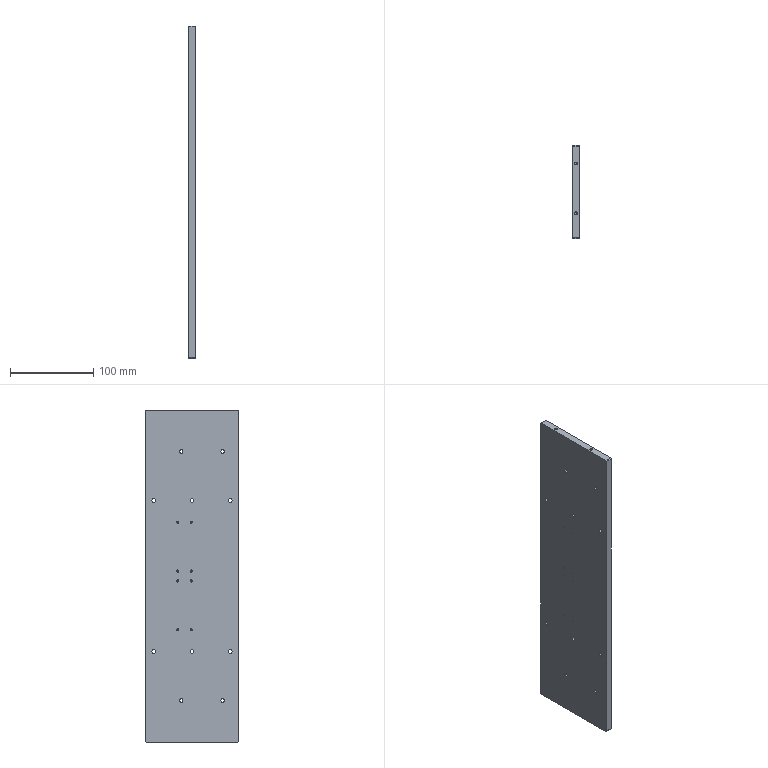Part | NX | 1 solid | 56 faces | box 8 x 112 x 400 mm | volume 355078 mm3 | cylinder 32 | plane 16 | cone 8 | commonest cylinder face diameters 2.5 x8 3.3 x8 4.5 x6 8 x6 4.2 x4
STEP:
#1=CARTESIAN_POINT('',(4.,1.,-4.75));
#2=VERTEX_POINT('',#1);
#3=CARTESIAN_POINT('',(4.,1.,-6.));
#4=DIRECTION('',(-1.,0.,0.));
#5=DIRECTION('',(0.,0.,1.));
#6=AXIS2_PLACEMENT_3D('',#3,#4,#5);
#7=CIRCLE('',#6,1.25);
#8=EDGE_CURVE('',#2,#2,#7,.T.);
#9=ORIENTED_EDGE('',*,*,#8,.T.);
#10=EDGE_LOOP('',(#9));
#11=FACE_BOUND('',#10,.T.);
#12=CARTESIAN_POINT('',(4.,17.,-4.75));
#13=VERTEX_POINT('',#12);
#14=CARTESIAN_POINT('',(4.,17.,-6.));
#15=DIRECTION('',(-1.,0.,0.));
#16=DIRECTION('',(0.,0.,1.));
#17=AXIS2_PLACEMENT_3D('',#14,#15,#16);
#18=CIRCLE('',#17,1.25);
#19=EDGE_CURVE('',#13,#13,#18,.T.);
#20=ORIENTED_EDGE('',*,*,#19,.T.);
#21=EDGE_LOOP('',(#20));
#22=FACE_BOUND('',#21,.T.);
#23=CARTESIAN_POINT('',(4.,17.,7.25));
#24=VERTEX_POINT('',#23);
#25=CARTESIAN_POINT('',(4.,17.,6.));
#26=DIRECTION('',(-1.,0.,0.));
#27=DIRECTION('',(0.,0.,1.));
#28=AXIS2_PLACEMENT_3D('',#25,#26,#27);
#29=CIRCLE('',#28,1.25);
#30=EDGE_CURVE('',#24,#24,#29,.T.);
#31=ORIENTED_EDGE('',*,*,#30,.T.);
#32=EDGE_LOOP('',(#31));
#33=FACE_BOUND('',#32,.T.);
#34=CARTESIAN_POINT('',(4.,1.,7.25));
#35=VERTEX_POINT('',#34);
#36=CARTESIAN_POINT('',(4.,1.,6.));
#37=DIRECTION('',(-1.,0.,0.));
#38=DIRECTION('',(0.,0.,1.));
#39=AXIS2_PLACEMENT_3D('',#36,#37,#38);
#40=CIRCLE('',#39,1.25);
#41=EDGE_CURVE('',#35,#35,#40,.T.);
#42=ORIENTED_EDGE('',*,*,#41,.T.);
#43=EDGE_LOOP('',(#42));
#44=FACE_BOUND('',#43,.T.);
#45=CARTESIAN_POINT('',(4.,17.,-63.75));
#46=VERTEX_POINT('',#45);
#47=CARTESIAN_POINT('',(4.,17.,-65.));
#48=DIRECTION('',(-1.,0.,0.));
#49=DIRECTION('',(0.,0.,1.));
#50=AXIS2_PLACEMENT_3D('',#47,#48,#49);
#51=CIRCLE('',#50,1.25);
#52=EDGE_CURVE('',#46,#46,#51,.T.);
#53=ORIENTED_EDGE('',*,*,#52,.T.);
#54=EDGE_LOOP('',(#53));
#55=FACE_BOUND('',#54,.T.);
#56=CARTESIAN_POINT('',(4.,1.,-63.75));
#57=VERTEX_POINT('',#56);
#58=CARTESIAN_POINT('',(4.,1.,-65.));
#59=DIRECTION('',(-1.,0.,0.));
#60=DIRECTION('',(0.,0.,1.));
#61=AXIS2_PLACEMENT_3D('',#58,#59,#60);
#62=CIRCLE('',#61,1.25);
#63=EDGE_CURVE('',#57,#57,#62,.T.);
#64=ORIENTED_EDGE('',*,*,#63,.T.);
#65=EDGE_LOOP('',(#64));
#66=FACE_BOUND('',#65,.T.);
#67=CARTESIAN_POINT('',(4.,1.,66.25));
#68=VERTEX_POINT('',#67);
#69=CARTESIAN_POINT('',(4.,1.,65.));
#70=DIRECTION('',(-1.,0.,0.));
#71=DIRECTION('',(0.,0.,1.));
#72=AXIS2_PLACEMENT_3D('',#69,#70,#71);
#73=CIRCLE('',#72,1.25);
#74=EDGE_CURVE('',#68,#68,#73,.T.);
#75=ORIENTED_EDGE('',*,*,#74,.T.);
#76=EDGE_LOOP('',(#75));
#77=FACE_BOUND('',#76,.T.);
#78=CARTESIAN_POINT('',(4.,17.,66.25));
#79=VERTEX_POINT('',#78);
#80=CARTESIAN_POINT('',(4.,17.,65.));
#81=DIRECTION('',(-1.,0.,0.));
#82=DIRECTION('',(0.,0.,1.));
#83=AXIS2_PLACEMENT_3D('',#80,#81,#82);
#84=CIRCLE('',#83,1.25);
#85=EDGE_CURVE('',#79,#79,#84,.T.);
#86=ORIENTED_EDGE('',*,*,#85,.T.);
#87=EDGE_LOOP('',(#86));
#88=FACE_BOUND('',#87,.T.);
#89=CARTESIAN_POINT('',(4.,46.,87.));
#90=VERTEX_POINT('',#89);
#91=CARTESIAN_POINT('',(4.,46.,91.));
#92=DIRECTION('',(1.,0.,0.));
#93=DIRECTION('',(0.,0.,-1.));
#94=AXIS2_PLACEMENT_3D('',#91,#92,#93);
#95=CIRCLE('',#94,4.);
#96=EDGE_CURVE('',#90,#90,#95,.T.);
#97=ORIENTED_EDGE('',*,*,#96,.F.);
#98=EDGE_LOOP('',(#97));
#99=FACE_BOUND('',#98,.T.);
#100=CARTESIAN_POINT('',(4.,0.,87.));
#101=VERTEX_POINT('',#100);
#102=CARTESIAN_POINT('',(4.,0.,91.));
#103=DIRECTION('',(1.,0.,0.));
#104=DIRECTION('',(0.,0.,-1.));
#105=AXIS2_PLACEMENT_3D('',#102,#103,#104);
#106=CIRCLE('',#105,4.);
#107=EDGE_CURVE('',#101,#101,#106,.T.);
#108=ORIENTED_EDGE('',*,*,#107,.F.);
#109=EDGE_LOOP('',(#108));
#110=FACE_BOUND('',#109,.T.);
#111=CARTESIAN_POINT('',(4.,-46.,87.));
#112=VERTEX_POINT('',#111);
#113=CARTESIAN_POINT('',(4.,-46.,91.));
#114=DIRECTION('',(1.,0.,0.));
#115=DIRECTION('',(0.,0.,-1.));
#116=AXIS2_PLACEMENT_3D('',#113,#114,#115);
#117=CIRCLE('',#116,4.);
#118=EDGE_CURVE('',#112,#112,#117,.T.);
#119=ORIENTED_EDGE('',*,*,#118,.F.);
#120=EDGE_LOOP('',(#119));
#121=FACE_BOUND('',#120,.T.);
#122=CARTESIAN_POINT('',(4.,46.,-95.));
#123=VERTEX_POINT('',#122);
#124=CARTESIAN_POINT('',(4.,46.,-91.));
#125=DIRECTION('',(1.,0.,0.));
#126=DIRECTION('',(0.,0.,-1.));
#127=AXIS2_PLACEMENT_3D('',#124,#125,#126);
#128=CIRCLE('',#127,4.);
#129=EDGE_CURVE('',#123,#123,#128,.T.);
#130=ORIENTED_EDGE('',*,*,#129,.F.);
#131=EDGE_LOOP('',(#130));
#132=FACE_BOUND('',#131,.T.);
#133=CARTESIAN_POINT('',(4.,0.,-95.));
#134=VERTEX_POINT('',#133);
#135=CARTESIAN_POINT('',(4.,0.,-91.));
#136=DIRECTION('',(1.,0.,0.));
#137=DIRECTION('',(0.,0.,-1.));
#138=AXIS2_PLACEMENT_3D('',#135,#136,#137);
#139=CIRCLE('',#138,4.);
#140=EDGE_CURVE('',#134,#134,#139,.T.);
#141=ORIENTED_EDGE('',*,*,#140,.F.);
#142=EDGE_LOOP('',(#141));
#143=FACE_BOUND('',#142,.T.);
#144=CARTESIAN_POINT('',(4.,-46.,-95.));
#145=VERTEX_POINT('',#144);
#146=CARTESIAN_POINT('',(4.,-46.,-91.));
#147=DIRECTION('',(1.,0.,0.));
#148=DIRECTION('',(0.,0.,-1.));
#149=AXIS2_PLACEMENT_3D('',#146,#147,#148);
#150=CIRCLE('',#149,4.);
#151=EDGE_CURVE('',#145,#145,#150,.T.);
#152=ORIENTED_EDGE('',*,*,#151,.F.);
#153=EDGE_LOOP('',(#152));
#154=FACE_BOUND('',#153,.T.);
#155=CARTESIAN_POINT('',(4.,13.,-147.9));
#156=VERTEX_POINT('',#155);
#157=CARTESIAN_POINT('',(4.,13.,-150.));
#158=DIRECTION('',(-1.,0.,0.));
#159=DIRECTION('',(0.,0.,1.));
#160=AXIS2_PLACEMENT_3D('',#157,#158,#159);
#161=CIRCLE('',#160,2.1);
#162=EDGE_CURVE('',#156,#156,#161,.T.);
#163=ORIENTED_EDGE('',*,*,#162,.T.);
#164=EDGE_LOOP('',(#163));
#165=FACE_BOUND('',#164,.T.);
#166=CARTESIAN_POINT('',(4.,-37.,152.1));
#167=VERTEX_POINT('',#166);
#168=CARTESIAN_POINT('',(4.,-37.,150.));
#169=DIRECTION('',(-1.,0.,0.));
#170=DIRECTION('',(0.,0.,1.));
#171=AXIS2_PLACEMENT_3D('',#168,#169,#170);
#172=CIRCLE('',#171,2.1);
#173=EDGE_CURVE('',#167,#167,#172,.T.);
#174=ORIENTED_EDGE('',*,*,#173,.T.);
#175=EDGE_LOOP('',(#174));
#176=FACE_BOUND('',#175,.T.);
#177=CARTESIAN_POINT('',(4.,-37.,-147.9));
#178=VERTEX_POINT('',#177);
#179=CARTESIAN_POINT('',(4.,-37.,-150.));
#180=DIRECTION('',(-1.,0.,0.));
#181=DIRECTION('',(0.,0.,1.));
#182=AXIS2_PLACEMENT_3D('',#179,#180,#181);
#183=CIRCLE('',#182,2.1);
#184=EDGE_CURVE('',#178,#178,#183,.T.);
#185=ORIENTED_EDGE('',*,*,#184,.T.);
#186=EDGE_LOOP('',(#185));
#187=FACE_BOUND('',#186,.T.);
#188=CARTESIAN_POINT('',(4.,13.,152.1));
#189=VERTEX_POINT('',#188);
#190=CARTESIAN_POINT('',(4.,13.,150.));
#191=DIRECTION('',(-1.,0.,0.));
#192=DIRECTION('',(0.,0.,1.));
#193=AXIS2_PLACEMENT_3D('',#190,#191,#192);
#194=CIRCLE('',#193,2.1);
#195=EDGE_CURVE('',#189,#189,#194,.T.);
#196=ORIENTED_EDGE('',*,*,#195,.T.);
#197=EDGE_LOOP('',(#196));
#198=FACE_BOUND('',#197,.T.);
#199=CARTESIAN_POINT('',(4.,56.,199.));
#200=VERTEX_POINT('',#199);
#201=CARTESIAN_POINT('',(4.,56.,-199.));
#202=VERTEX_POINT('',#201);
#203=CARTESIAN_POINT('',(4.,56.,200.));
#204=DIRECTION('',(0.,0.,-1.));
#205=VECTOR('',#204,1000.);
#206=LINE('',#203,#205);
#207=EDGE_CURVE('',#200,#202,#206,.T.);
#208=ORIENTED_EDGE('',*,*,#207,.F.);
#209=CARTESIAN_POINT('',(4.,55.,200.));
#210=VERTEX_POINT('',#209);
#211=CARTESIAN_POINT('',(4.,55.,200.));
#212=DIRECTION('',(0.,-0.7071,0.7071));
#213=VECTOR('',#212,1000.);
#214=LINE('',#211,#213);
#215=EDGE_CURVE('',#200,#210,#214,.T.);
#216=ORIENTED_EDGE('',*,*,#215,.T.);
#217=CARTESIAN_POINT('',(4.,-55.,200.));
#218=VERTEX_POINT('',#217);
#219=CARTESIAN_POINT('',(4.,56.,200.));
#220=DIRECTION('',(0.,1.,0.));
#221=VECTOR('',#220,1000.);
#222=LINE('',#219,#221);
#223=EDGE_CURVE('',#218,#210,#222,.T.);
#224=ORIENTED_EDGE('',*,*,#223,.F.);
#225=CARTESIAN_POINT('',(4.,-56.,199.));
#226=VERTEX_POINT('',#225);
#227=CARTESIAN_POINT('',(4.,-55.,200.));
#228=DIRECTION('',(0.,-0.7071,-0.7071));
#229=VECTOR('',#228,1000.);
#230=LINE('',#227,#229);
#231=EDGE_CURVE('',#218,#226,#230,.T.);
#232=ORIENTED_EDGE('',*,*,#231,.T.);
#233=CARTESIAN_POINT('',(4.,-56.,-199.));
#234=VERTEX_POINT('',#233);
#235=CARTESIAN_POINT('',(4.,-56.,200.));
#236=DIRECTION('',(0.,0.,-1.));
#237=VECTOR('',#236,1000.);
#238=LINE('',#235,#237);
#239=EDGE_CURVE('',#226,#234,#238,.T.);
#240=ORIENTED_EDGE('',*,*,#239,.T.);
#241=CARTESIAN_POINT('',(4.,-55.,-200.));
#242=VERTEX_POINT('',#241);
#243=CARTESIAN_POINT('',(4.,-56.,-199.));
#244=DIRECTION('',(0.,-0.7071,0.7071));
#245=VECTOR('',#244,1000.);
#246=LINE('',#243,#245);
#247=EDGE_CURVE('',#234,#242,#246,.F.);
#248=ORIENTED_EDGE('',*,*,#247,.T.);
#249=CARTESIAN_POINT('',(4.,55.,-200.));
#250=VERTEX_POINT('',#249);
#251=CARTESIAN_POINT('',(4.,56.,-200.));
#252=DIRECTION('',(0.,1.,0.));
#253=VECTOR('',#252,1000.);
#254=LINE('',#251,#253);
#255=EDGE_CURVE('',#242,#250,#254,.T.);
#256=ORIENTED_EDGE('',*,*,#255,.T.);
#257=CARTESIAN_POINT('',(4.,56.,-199.));
#258=DIRECTION('',(0.,-0.7071,-0.7071));
#259=VECTOR('',#258,1000.);
#260=LINE('',#257,#259);
#261=EDGE_CURVE('',#250,#202,#260,.F.);
#262=ORIENTED_EDGE('',*,*,#261,.T.);
#263=EDGE_LOOP('',(#208,#216,#224,#232,#240,#248,#256,#262));
#264=FACE_BOUND('',#263,.T.);
#265=CARTESIAN_POINT('',(4.,56.,200.));
#266=DIRECTION('',(-1.,0.,0.));
#267=DIRECTION('',(0.,-1.,0.));
#268=AXIS2_PLACEMENT_3D('',#265,#266,#267);
#269=PLANE('',#268);
#270=ADVANCED_FACE('',(#11,#22,#33,#44,#55,#66,#77,#88,#99,#110,#121,#132,#143,#154,#165,#176,#187,#198,#264),#269,.F.);
#271=CARTESIAN_POINT('',(0.,56.,61.65));
#272=VERTEX_POINT('',#271);
#273=CARTESIAN_POINT('',(0.,56.,60.));
#274=DIRECTION('',(0.,1.,0.));
#275=DIRECTION('',(0.,0.,1.));
#276=AXIS2_PLACEMENT_3D('',#273,#274,#275);
#277=CIRCLE('',#276,1.65);
#278=EDGE_CURVE('',#272,#272,#277,.T.);
#279=ORIENTED_EDGE('',*,*,#278,.F.);
#280=EDGE_LOOP('',(#279));
#281=FACE_BOUND('',#280,.T.);
#282=CARTESIAN_POINT('',(0.,56.,181.65));
#283=VERTEX_POINT('',#282);
#284=CARTESIAN_POINT('',(0.,56.,180.));
#285=DIRECTION('',(0.,1.,0.));
#286=DIRECTION('',(0.,0.,1.));
#287=AXIS2_PLACEMENT_3D('',#284,#285,#286);
#288=CIRCLE('',#287,1.65);
#289=EDGE_CURVE('',#283,#283,#288,.T.);
#290=ORIENTED_EDGE('',*,*,#289,.F.);
#291=EDGE_LOOP('',(#290));
#292=FACE_BOUND('',#291,.T.);
#293=CARTESIAN_POINT('',(0.,56.,-58.35));
#294=VERTEX_POINT('',#293);
#295=CARTESIAN_POINT('',(0.,56.,-60.));
#296=DIRECTION('',(0.,1.,0.));
#297=DIRECTION('',(0.,0.,1.));
#298=AXIS2_PLACEMENT_3D('',#295,#296,#297);
#299=CIRCLE('',#298,1.65);
#300=EDGE_CURVE('',#294,#294,#299,.T.);
#301=ORIENTED_EDGE('',*,*,#300,.F.);
#302=EDGE_LOOP('',(#301));
#303=FACE_BOUND('',#302,.T.);
#304=CARTESIAN_POINT('',(0.,56.,-178.35));
#305=VERTEX_POINT('',#304);
#306=CARTESIAN_POINT('',(0.,56.,-180.));
#307=DIRECTION('',(0.,1.,0.));
#308=DIRECTION('',(0.,0.,1.));
#309=AXIS2_PLACEMENT_3D('',#306,#307,#308);
#310=CIRCLE('',#309,1.65);
#311=EDGE_CURVE('',#305,#305,#310,.T.);
#312=ORIENTED_EDGE('',*,*,#311,.F.);
#313=EDGE_LOOP('',(#312));
#314=FACE_BOUND('',#313,.T.);
#315=CARTESIAN_POINT('',(-4.,56.,199.));
#316=VERTEX_POINT('',#315);
#317=CARTESIAN_POINT('',(-4.,56.,-199.));
#318=VERTEX_POINT('',#317);
#319=CARTESIAN_POINT('',(-4.,56.,200.));
#320=DIRECTION('',(0.,0.,-1.));
#321=VECTOR('',#320,1000.);
#322=LINE('',#319,#321);
#323=EDGE_CURVE('',#316,#318,#322,.T.);
#324=ORIENTED_EDGE('',*,*,#323,.F.);
#325=CARTESIAN_POINT('',(4.,56.,199.));
#326=DIRECTION('',(1.,0.,0.));
#327=VECTOR('',#326,1000.);
#328=LINE('',#325,#327);
#329=EDGE_CURVE('',#316,#200,#328,.T.);
#330=ORIENTED_EDGE('',*,*,#329,.T.);
#331=ORIENTED_EDGE('',*,*,#207,.T.);
#332=CARTESIAN_POINT('',(-4.,56.,-199.));
#333=DIRECTION('',(-1.,0.,0.));
#334=VECTOR('',#333,1000.);
#335=LINE('',#332,#334);
#336=EDGE_CURVE('',#202,#318,#335,.T.);
#337=ORIENTED_EDGE('',*,*,#336,.T.);
#338=EDGE_LOOP('',(#324,#330,#331,#337));
#339=FACE_BOUND('',#338,.T.);
#340=CARTESIAN_POINT('',(-4.,56.,200.));
#341=DIRECTION('',(0.,-1.,0.));
#342=DIRECTION('',(0.,0.,-1.));
#343=AXIS2_PLACEMENT_3D('',#340,#341,#342);
#344=PLANE('',#343);
#345=ADVANCED_FACE('',(#281,#292,#303,#314,#339),#344,.F.);
#346=CARTESIAN_POINT('',(-4.,1.,-4.75));
#347=VERTEX_POINT('',#346);
#348=CARTESIAN_POINT('',(-4.,1.,-6.));
#349=DIRECTION('',(-1.,0.,0.));
#350=DIRECTION('',(0.,0.,1.));
#351=AXIS2_PLACEMENT_3D('',#348,#349,#350);
#352=CIRCLE('',#351,1.25);
#353=EDGE_CURVE('',#347,#347,#352,.T.);
#354=ORIENTED_EDGE('',*,*,#353,.F.);
#355=EDGE_LOOP('',(#354));
#356=FACE_BOUND('',#355,.T.);
#357=CARTESIAN_POINT('',(-4.,17.,-4.75));
#358=VERTEX_POINT('',#357);
#359=CARTESIAN_POINT('',(-4.,17.,-6.));
#360=DIRECTION('',(-1.,0.,0.));
#361=DIRECTION('',(0.,0.,1.));
#362=AXIS2_PLACEMENT_3D('',#359,#360,#361);
#363=CIRCLE('',#362,1.25);
#364=EDGE_CURVE('',#358,#358,#363,.T.);
#365=ORIENTED_EDGE('',*,*,#364,.F.);
#366=EDGE_LOOP('',(#365));
#367=FACE_BOUND('',#366,.T.);
#368=CARTESIAN_POINT('',(-4.,17.,7.25));
#369=VERTEX_POINT('',#368);
#370=CARTESIAN_POINT('',(-4.,17.,6.));
#371=DIRECTION('',(-1.,0.,0.));
#372=DIRECTION('',(0.,0.,1.));
#373=AXIS2_PLACEMENT_3D('',#370,#371,#372);
#374=CIRCLE('',#373,1.25);
#375=EDGE_CURVE('',#369,#369,#374,.T.);
#376=ORIENTED_EDGE('',*,*,#375,.F.);
#377=EDGE_LOOP('',(#376));
#378=FACE_BOUND('',#377,.T.);
#379=CARTESIAN_POINT('',(-4.,1.,7.25));
#380=VERTEX_POINT('',#379);
#381=CARTESIAN_POINT('',(-4.,1.,6.));
#382=DIRECTION('',(-1.,0.,0.));
#383=DIRECTION('',(0.,0.,1.));
#384=AXIS2_PLACEMENT_3D('',#381,#382,#383);
#385=CIRCLE('',#384,1.25);
#386=EDGE_CURVE('',#380,#380,#385,.T.);
#387=ORIENTED_EDGE('',*,*,#386,.F.);
#388=EDGE_LOOP('',(#387));
#389=FACE_BOUND('',#388,.T.);
#390=CARTESIAN_POINT('',(-4.,17.,-63.75));
#391=VERTEX_POINT('',#390);
#392=CARTESIAN_POINT('',(-4.,17.,-65.));
#393=DIRECTION('',(-1.,0.,0.));
#394=DIRECTION('',(0.,0.,1.));
#395=AXIS2_PLACEMENT_3D('',#392,#393,#394);
#396=CIRCLE('',#395,1.25);
#397=EDGE_CURVE('',#391,#391,#396,.T.);
#398=ORIENTED_EDGE('',*,*,#397,.F.);
#399=EDGE_LOOP('',(#398));
#400=FACE_BOUND('',#399,.T.);
#401=CARTESIAN_POINT('',(-4.,1.,-63.75));
#402=VERTEX_POINT('',#401);
#403=CARTESIAN_POINT('',(-4.,1.,-65.));
#404=DIRECTION('',(-1.,0.,0.));
#405=DIRECTION('',(0.,0.,1.));
#406=AXIS2_PLACEMENT_3D('',#403,#404,#405);
#407=CIRCLE('',#406,1.25);
#408=EDGE_CURVE('',#402,#402,#407,.T.);
#409=ORIENTED_EDGE('',*,*,#408,.F.);
#410=EDGE_LOOP('',(#409));
#411=FACE_BOUND('',#410,.T.);
#412=CARTESIAN_POINT('',(-4.,1.,66.25));
#413=VERTEX_POINT('',#412);
#414=CARTESIAN_POINT('',(-4.,1.,65.));
#415=DIRECTION('',(-1.,0.,0.));
#416=DIRECTION('',(0.,0.,1.));
#417=AXIS2_PLACEMENT_3D('',#414,#415,#416);
#418=CIRCLE('',#417,1.25);
#419=EDGE_CURVE('',#413,#413,#418,.T.);
#420=ORIENTED_EDGE('',*,*,#419,.F.);
#421=EDGE_LOOP('',(#420));
#422=FACE_BOUND('',#421,.T.);
#423=CARTESIAN_POINT('',(-4.,17.,66.25));
#424=VERTEX_POINT('',#423);
#425=CARTESIAN_POINT('',(-4.,17.,65.));
#426=DIRECTION('',(-1.,0.,0.));
#427=DIRECTION('',(0.,0.,1.));
#428=AXIS2_PLACEMENT_3D('',#425,#426,#427);
#429=CIRCLE('',#428,1.25);
#430=EDGE_CURVE('',#424,#424,#429,.T.);
#431=ORIENTED_EDGE('',*,*,#430,.F.);
#432=EDGE_LOOP('',(#431));
#433=FACE_BOUND('',#432,.T.);
#434=CARTESIAN_POINT('',(-4.,46.,88.75));
#435=VERTEX_POINT('',#434);
#436=CARTESIAN_POINT('',(-4.,46.,91.));
#437=DIRECTION('',(1.,0.,0.));
#438=DIRECTION('',(0.,0.,-1.));
#439=AXIS2_PLACEMENT_3D('',#436,#437,#438);
#440=CIRCLE('',#439,2.25);
#441=EDGE_CURVE('',#435,#435,#440,.T.);
#442=ORIENTED_EDGE('',*,*,#441,.T.);
#443=EDGE_LOOP('',(#442));
#444=FACE_BOUND('',#443,.T.);
#445=CARTESIAN_POINT('',(-4.,0.,88.75));
#446=VERTEX_POINT('',#445);
#447=CARTESIAN_POINT('',(-4.,0.,91.));
#448=DIRECTION('',(1.,0.,0.));
#449=DIRECTION('',(0.,0.,-1.));
#450=AXIS2_PLACEMENT_3D('',#447,#448,#449);
#451=CIRCLE('',#450,2.25);
#452=EDGE_CURVE('',#446,#446,#451,.T.);
#453=ORIENTED_EDGE('',*,*,#452,.T.);
#454=EDGE_LOOP('',(#453));
#455=FACE_BOUND('',#454,.T.);
#456=CARTESIAN_POINT('',(-4.,-46.,88.75));
#457=VERTEX_POINT('',#456);
#458=CARTESIAN_POINT('',(-4.,-46.,91.));
#459=DIRECTION('',(1.,0.,0.));
#460=DIRECTION('',(0.,0.,-1.));
#461=AXIS2_PLACEMENT_3D('',#458,#459,#460);
#462=CIRCLE('',#461,2.25);
#463=EDGE_CURVE('',#457,#457,#462,.T.);
#464=ORIENTED_EDGE('',*,*,#463,.T.);
#465=EDGE_LOOP('',(#464));
#466=FACE_BOUND('',#465,.T.);
#467=CARTESIAN_POINT('',(-4.,46.,-93.25));
#468=VERTEX_POINT('',#467);
#469=CARTESIAN_POINT('',(-4.,46.,-91.));
#470=DIRECTION('',(1.,0.,0.));
#471=DIRECTION('',(0.,0.,-1.));
#472=AXIS2_PLACEMENT_3D('',#469,#470,#471);
#473=CIRCLE('',#472,2.25);
#474=EDGE_CURVE('',#468,#468,#473,.T.);
#475=ORIENTED_EDGE('',*,*,#474,.T.);
#476=EDGE_LOOP('',(#475));
#477=FACE_BOUND('',#476,.T.);
#478=CARTESIAN_POINT('',(-4.,0.,-93.25));
#479=VERTEX_POINT('',#478);
#480=CARTESIAN_POINT('',(-4.,0.,-91.));
#481=DIRECTION('',(1.,0.,0.));
#482=DIRECTION('',(0.,0.,-1.));
#483=AXIS2_PLACEMENT_3D('',#480,#481,#482);
#484=CIRCLE('',#483,2.25);
#485=EDGE_CURVE('',#479,#479,#484,.T.);
#486=ORIENTED_EDGE('',*,*,#485,.T.);
#487=EDGE_LOOP('',(#486));
#488=FACE_BOUND('',#487,.T.);
#489=CARTESIAN_POINT('',(-4.,-46.,-93.25));
#490=VERTEX_POINT('',#489);
#491=CARTESIAN_POINT('',(-4.,-46.,-91.));
#492=DIRECTION('',(1.,0.,0.));
#493=DIRECTION('',(0.,0.,-1.));
#494=AXIS2_PLACEMENT_3D('',#491,#492,#493);
#495=CIRCLE('',#494,2.25);
#496=EDGE_CURVE('',#490,#490,#495,.T.);
#497=ORIENTED_EDGE('',*,*,#496,.T.);
#498=EDGE_LOOP('',(#497));
#499=FACE_BOUND('',#498,.T.);
#500=CARTESIAN_POINT('',(-4.,13.,-147.9));
#501=VERTEX_POINT('',#500);
#502=CARTESIAN_POINT('',(-4.,13.,-150.));
#503=DIRECTION('',(-1.,0.,0.));
#504=DIRECTION('',(0.,0.,1.));
#505=AXIS2_PLACEMENT_3D('',#502,#503,#504);
#506=CIRCLE('',#505,2.1);
#507=EDGE_CURVE('',#501,#501,#506,.T.);
#508=ORIENTED_EDGE('',*,*,#507,.F.);
#509=EDGE_LOOP('',(#508));
#510=FACE_BOUND('',#509,.T.);
#511=CARTESIAN_POINT('',(-4.,-37.,152.1));
#512=VERTEX_POINT('',#511);
#513=CARTESIAN_POINT('',(-4.,-37.,150.));
#514=DIRECTION('',(-1.,0.,0.));
#515=DIRECTION('',(0.,0.,1.));
#516=AXIS2_PLACEMENT_3D('',#513,#514,#515);
#517=CIRCLE('',#516,2.1);
#518=EDGE_CURVE('',#512,#512,#517,.T.);
#519=ORIENTED_EDGE('',*,*,#518,.F.);
#520=EDGE_LOOP('',(#519));
#521=FACE_BOUND('',#520,.T.);
#522=CARTESIAN_POINT('',(-4.,-37.,-147.9));
#523=VERTEX_POINT('',#522);
#524=CARTESIAN_POINT('',(-4.,-37.,-150.));
#525=DIRECTION('',(-1.,0.,0.));
#526=DIRECTION('',(0.,0.,1.));
#527=AXIS2_PLACEMENT_3D('',#524,#525,#526);
#528=CIRCLE('',#527,2.1);
#529=EDGE_CURVE('',#523,#523,#528,.T.);
#530=ORIENTED_EDGE('',*,*,#529,.F.);
#531=EDGE_LOOP('',(#530));
#532=FACE_BOUND('',#531,.T.);
#533=CARTESIAN_POINT('',(-4.,13.,152.1));
#534=VERTEX_POINT('',#533);
#535=CARTESIAN_POINT('',(-4.,13.,150.));
#536=DIRECTION('',(-1.,0.,0.));
#537=DIRECTION('',(0.,0.,1.));
#538=AXIS2_PLACEMENT_3D('',#535,#536,#537);
#539=CIRCLE('',#538,2.1);
#540=EDGE_CURVE('',#534,#534,#539,.T.);
#541=ORIENTED_EDGE('',*,*,#540,.F.);
#542=EDGE_LOOP('',(#541));
#543=FACE_BOUND('',#542,.T.);
#544=CARTESIAN_POINT('',(-4.,55.,200.));
#545=VERTEX_POINT('',#544);
#546=CARTESIAN_POINT('',(-4.,-55.,200.));
#547=VERTEX_POINT('',#546);
#548=CARTESIAN_POINT('',(-4.,56.,200.));
#549=DIRECTION('',(0.,-1.,0.));
#550=VECTOR('',#549,1000.);
#551=LINE('',#548,#550);
#552=EDGE_CURVE('',#545,#547,#551,.T.);
#553=ORIENTED_EDGE('',*,*,#552,.F.);
#554=CARTESIAN_POINT('',(-4.,55.,200.));
#555=DIRECTION('',(0.,0.7071,-0.7071));
#556=VECTOR('',#555,1000.);
#557=LINE('',#554,#556);
#558=EDGE_CURVE('',#545,#316,#557,.T.);
#559=ORIENTED_EDGE('',*,*,#558,.T.);
#560=ORIENTED_EDGE('',*,*,#323,.T.);
#561=CARTESIAN_POINT('',(-4.,55.,-200.));
#562=VERTEX_POINT('',#561);
#563=CARTESIAN_POINT('',(-4.,56.,-199.));
#564=DIRECTION('',(0.,0.7071,0.7071));
#565=VECTOR('',#564,1000.);
#566=LINE('',#563,#565);
#567=EDGE_CURVE('',#318,#562,#566,.F.);
#568=ORIENTED_EDGE('',*,*,#567,.T.);
#569=CARTESIAN_POINT('',(-4.,-55.,-200.));
#570=VERTEX_POINT('',#569);
#571=CARTESIAN_POINT('',(-4.,56.,-200.));
#572=DIRECTION('',(0.,-1.,0.));
#573=VECTOR('',#572,1000.);
#574=LINE('',#571,#573);
#575=EDGE_CURVE('',#562,#570,#574,.T.);
#576=ORIENTED_EDGE('',*,*,#575,.T.);
#577=CARTESIAN_POINT('',(-4.,-56.,-199.));
#578=VERTEX_POINT('',#577);
#579=CARTESIAN_POINT('',(-4.,-56.,-199.));
#580=DIRECTION('',(0.,0.7071,-0.7071));
#581=VECTOR('',#580,1000.);
#582=LINE('',#579,#581);
#583=EDGE_CURVE('',#570,#578,#582,.F.);
#584=ORIENTED_EDGE('',*,*,#583,.T.);
#585=CARTESIAN_POINT('',(-4.,-56.,199.));
#586=VERTEX_POINT('',#585);
#587=CARTESIAN_POINT('',(-4.,-56.,200.));
#588=DIRECTION('',(0.,0.,-1.));
#589=VECTOR('',#588,1000.);
#590=LINE('',#587,#589);
#591=EDGE_CURVE('',#586,#578,#590,.T.);
#592=ORIENTED_EDGE('',*,*,#591,.F.);
#593=CARTESIAN_POINT('',(-4.,-55.,200.));
#594=DIRECTION('',(0.,0.7071,0.7071));
#595=VECTOR('',#594,1000.);
#596=LINE('',#593,#595);
#597=EDGE_CURVE('',#586,#547,#596,.T.);
#598=ORIENTED_EDGE('',*,*,#597,.T.);
#599=EDGE_LOOP('',(#553,#559,#560,#568,#576,#584,#592,#598));
#600=FACE_BOUND('',#599,.T.);
#601=CARTESIAN_POINT('',(-4.,56.,200.));
#602=DIRECTION('',(1.,0.,0.));
#603=DIRECTION('',(0.,1.,0.));
#604=AXIS2_PLACEMENT_3D('',#601,#602,#603);
#605=PLANE('',#604);
#606=ADVANCED_FACE('',(#356,#367,#378,#389,#400,#411,#422,#433,#444,#455,#466,#477,#488,#499,#510,#521,#532,#543,#600),#605,.F.);
#607=ORIENTED_EDGE('',*,*,#239,.F.);
#608=CARTESIAN_POINT('',(-4.,-56.,199.));
#609=DIRECTION('',(-1.,0.,0.));
#610=VECTOR('',#609,1000.);
#611=LINE('',#608,#610);
#612=EDGE_CURVE('',#226,#586,#611,.T.);
#613=ORIENTED_EDGE('',*,*,#612,.T.);
#614=ORIENTED_EDGE('',*,*,#591,.T.);
#615=CARTESIAN_POINT('',(-4.,-56.,-199.));
#616=DIRECTION('',(1.,0.,0.));
#617=VECTOR('',#616,1000.);
#618=LINE('',#615,#617);
#619=EDGE_CURVE('',#578,#234,#618,.T.);
#620=ORIENTED_EDGE('',*,*,#619,.T.);
#621=EDGE_LOOP('',(#607,#613,#614,#620));
#622=FACE_BOUND('',#621,.T.);
#623=CARTESIAN_POINT('',(-4.,-56.,200.));
#624=DIRECTION('',(0.,1.,0.));
#625=DIRECTION('',(0.,0.,1.));
#626=AXIS2_PLACEMENT_3D('',#623,#624,#625);
#627=PLANE('',#626);
#628=ADVANCED_FACE('',(#622),#627,.F.);
#629=CARTESIAN_POINT('',(1.65,34.,200.));
#630=VERTEX_POINT('',#629);
#631=CARTESIAN_POINT('',(0.,34.,200.));
#632=DIRECTION('',(0.,0.,1.));
#633=DIRECTION('',(1.,0.,0.));
#634=AXIS2_PLACEMENT_3D('',#631,#632,#633);
#635=CIRCLE('',#634,1.65);
#636=EDGE_CURVE('',#630,#630,#635,.T.);
#637=ORIENTED_EDGE('',*,*,#636,.F.);
#638=EDGE_LOOP('',(#637));
#639=FACE_BOUND('',#638,.T.);
#640=CARTESIAN_POINT('',(1.65,-26.,200.));
#641=VERTEX_POINT('',#640);
#642=CARTESIAN_POINT('',(0.,-26.,200.));
#643=DIRECTION('',(0.,0.,1.));
#644=DIRECTION('',(1.,0.,0.));
#645=AXIS2_PLACEMENT_3D('',#642,#643,#644);
#646=CIRCLE('',#645,1.65);
#647=EDGE_CURVE('',#641,#641,#646,.T.);
#648=ORIENTED_EDGE('',*,*,#647,.F.);
#649=EDGE_LOOP('',(#648));
#650=FACE_BOUND('',#649,.T.);
#651=ORIENTED_EDGE('',*,*,#223,.T.);
#652=CARTESIAN_POINT('',(-4.,55.,200.));
#653=DIRECTION('',(-1.,0.,0.));
#654=VECTOR('',#653,1000.);
#655=LINE('',#652,#654);
#656=EDGE_CURVE('',#210,#545,#655,.T.);
#657=ORIENTED_EDGE('',*,*,#656,.T.);
#658=ORIENTED_EDGE('',*,*,#552,.T.);
#659=CARTESIAN_POINT('',(4.,-55.,200.));
#660=DIRECTION('',(1.,0.,0.));
#661=VECTOR('',#660,1000.);
#662=LINE('',#659,#661);
#663=EDGE_CURVE('',#547,#218,#662,.T.);
#664=ORIENTED_EDGE('',*,*,#663,.T.);
#665=EDGE_LOOP('',(#651,#657,#658,#664));
#666=FACE_BOUND('',#665,.T.);
#667=CARTESIAN_POINT('',(0.,0.,200.));
#668=DIRECTION('',(0.,0.,1.));
#669=DIRECTION('',(1.,0.,0.));
#670=AXIS2_PLACEMENT_3D('',#667,#668,#669);
#671=PLANE('',#670);
#672=ADVANCED_FACE('',(#639,#650,#666),#671,.T.);
#673=CARTESIAN_POINT('',(-1.65,34.,-200.));
#674=VERTEX_POINT('',#673);
#675=CARTESIAN_POINT('',(0.,34.,-200.));
#676=DIRECTION('',(0.,0.,-1.));
#677=DIRECTION('',(-1.,0.,0.));
#678=AXIS2_PLACEMENT_3D('',#675,#676,#677);
#679=CIRCLE('',#678,1.65);
#680=EDGE_CURVE('',#674,#674,#679,.T.);
#681=ORIENTED_EDGE('',*,*,#680,.F.);
#682=EDGE_LOOP('',(#681));
#683=FACE_BOUND('',#682,.T.);
#684=CARTESIAN_POINT('',(-1.65,-26.,-200.));
#685=VERTEX_POINT('',#684);
#686=CARTESIAN_POINT('',(0.,-26.,-200.));
#687=DIRECTION('',(0.,0.,-1.));
#688=DIRECTION('',(-1.,0.,0.));
#689=AXIS2_PLACEMENT_3D('',#686,#687,#688);
#690=CIRCLE('',#689,1.65);
#691=EDGE_CURVE('',#685,#685,#690,.T.);
#692=ORIENTED_EDGE('',*,*,#691,.F.);
#693=EDGE_LOOP('',(#692));
#694=FACE_BOUND('',#693,.T.);
#695=ORIENTED_EDGE('',*,*,#255,.F.);
#696=CARTESIAN_POINT('',(0.,-55.,-200.));
#697=DIRECTION('',(-1.,0.,0.));
#698=VECTOR('',#697,1000.);
#699=LINE('',#696,#698);
#700=EDGE_CURVE('',#242,#570,#699,.T.);
#701=ORIENTED_EDGE('',*,*,#700,.T.);
#702=ORIENTED_EDGE('',*,*,#575,.F.);
#703=CARTESIAN_POINT('',(0.,55.,-200.));
#704=DIRECTION('',(1.,0.,0.));
#705=VECTOR('',#704,1000.);
#706=LINE('',#703,#705);
#707=EDGE_CURVE('',#562,#250,#706,.T.);
#708=ORIENTED_EDGE('',*,*,#707,.T.);
#709=EDGE_LOOP('',(#695,#701,#702,#708));
#710=FACE_BOUND('',#709,.T.);
#711=CARTESIAN_POINT('',(0.,0.,-200.));
#712=DIRECTION('',(0.,0.,1.));
#713=DIRECTION('',(1.,0.,0.));
#714=AXIS2_PLACEMENT_3D('',#711,#712,#713);
#715=PLANE('',#714);
#716=ADVANCED_FACE('',(#683,#694,#710),#715,.F.);
#717=CARTESIAN_POINT('',(0.,-26.,-189.009));
#718=VERTEX_POINT('',#717);
#719=VERTEX_LOOP('',#718);
#720=FACE_BOUND('',#719,.T.);
#721=CARTESIAN_POINT('',(-1.65,-26.,-190.));
#722=VERTEX_POINT('',#721);
#723=CARTESIAN_POINT('',(0.,-26.,-190.));
#724=DIRECTION('',(0.,0.,-1.));
#725=DIRECTION('',(-1.,0.,0.));
#726=AXIS2_PLACEMENT_3D('',#723,#724,#725);
#727=CIRCLE('',#726,1.65);
#728=EDGE_CURVE('',#722,#722,#727,.T.);
#729=ORIENTED_EDGE('',*,*,#728,.T.);
#730=EDGE_LOOP('',(#729));
#731=FACE_BOUND('',#730,.T.);
#732=CARTESIAN_POINT('',(0.,-26.,-190.));
#733=DIRECTION('',(0.,0.,-1.));
#734=DIRECTION('',(-1.,0.,0.));
#735=AXIS2_PLACEMENT_3D('',#732,#733,#734);
#736=CONICAL_SURFACE('',#735,1.65,1.03);
#737=ADVANCED_FACE('',(#720,#731),#736,.F.);
#738=ORIENTED_EDGE('',*,*,#728,.F.);
#739=EDGE_LOOP('',(#738));
#740=FACE_BOUND('',#739,.T.);
#741=ORIENTED_EDGE('',*,*,#691,.T.);
#742=EDGE_LOOP('',(#741));
#743=FACE_BOUND('',#742,.T.);
#744=CARTESIAN_POINT('',(0.,-26.,-200.));
#745=DIRECTION('',(0.,0.,-1.));
#746=DIRECTION('',(-1.,0.,0.));
#747=AXIS2_PLACEMENT_3D('',#744,#745,#746);
#748=CYLINDRICAL_SURFACE('',#747,1.65);
#749=ADVANCED_FACE('',(#740,#743),#748,.F.);
#750=CARTESIAN_POINT('',(0.,34.,-189.009));
#751=VERTEX_POINT('',#750);
#752=VERTEX_LOOP('',#751);
#753=FACE_BOUND('',#752,.T.);
#754=CARTESIAN_POINT('',(-1.65,34.,-190.));
#755=VERTEX_POINT('',#754);
#756=CARTESIAN_POINT('',(0.,34.,-190.));
#757=DIRECTION('',(0.,0.,-1.));
#758=DIRECTION('',(-1.,0.,0.));
#759=AXIS2_PLACEMENT_3D('',#756,#757,#758);
#760=CIRCLE('',#759,1.65);
#761=EDGE_CURVE('',#755,#755,#760,.T.);
#762=ORIENTED_EDGE('',*,*,#761,.T.);
#763=EDGE_LOOP('',(#762));
#764=FACE_BOUND('',#763,.T.);
#765=CARTESIAN_POINT('',(0.,34.,-190.));
#766=DIRECTION('',(0.,0.,-1.));
#767=DIRECTION('',(-1.,0.,0.));
#768=AXIS2_PLACEMENT_3D('',#765,#766,#767);
#769=CONICAL_SURFACE('',#768,1.65,1.03);
#770=ADVANCED_FACE('',(#753,#764),#769,.F.);
#771=ORIENTED_EDGE('',*,*,#761,.F.);
#772=EDGE_LOOP('',(#771));
#773=FACE_BOUND('',#772,.T.);
#774=ORIENTED_EDGE('',*,*,#680,.T.);
#775=EDGE_LOOP('',(#774));
#776=FACE_BOUND('',#775,.T.);
#777=CARTESIAN_POINT('',(0.,34.,-200.));
#778=DIRECTION('',(0.,0.,-1.));
#779=DIRECTION('',(-1.,0.,0.));
#780=AXIS2_PLACEMENT_3D('',#777,#778,#779);
#781=CYLINDRICAL_SURFACE('',#780,1.65);
#782=ADVANCED_FACE('',(#773,#776),#781,.F.);
#783=CARTESIAN_POINT('',(0.,40.009,-180.));
#784=VERTEX_POINT('',#783);
#785=VERTEX_LOOP('',#784);
#786=FACE_BOUND('',#785,.T.);
#787=CARTESIAN_POINT('',(0.,41.,-178.35));
#788=VERTEX_POINT('',#787);
#789=CARTESIAN_POINT('',(0.,41.,-180.));
#790=DIRECTION('',(0.,1.,0.));
#791=DIRECTION('',(0.,0.,1.));
#792=AXIS2_PLACEMENT_3D('',#789,#790,#791);
#793=CIRCLE('',#792,1.65);
#794=EDGE_CURVE('',#788,#788,#793,.T.);
#795=ORIENTED_EDGE('',*,*,#794,.T.);
#796=EDGE_LOOP('',(#795));
#797=FACE_BOUND('',#796,.T.);
#798=CARTESIAN_POINT('',(0.,41.,-180.));
#799=DIRECTION('',(0.,1.,0.));
#800=DIRECTION('',(0.,0.,1.));
#801=AXIS2_PLACEMENT_3D('',#798,#799,#800);
#802=CONICAL_SURFACE('',#801,1.65,1.03);
#803=ADVANCED_FACE('',(#786,#797),#802,.F.);
#804=ORIENTED_EDGE('',*,*,#794,.F.);
#805=EDGE_LOOP('',(#804));
#806=FACE_BOUND('',#805,.T.);
#807=ORIENTED_EDGE('',*,*,#311,.T.);
#808=EDGE_LOOP('',(#807));
#809=FACE_BOUND('',#808,.T.);
#810=CARTESIAN_POINT('',(0.,56.,-180.));
#811=DIRECTION('',(0.,1.,0.));
#812=DIRECTION('',(0.,0.,1.));
#813=AXIS2_PLACEMENT_3D('',#810,#811,#812);
#814=CYLINDRICAL_SURFACE('',#813,1.65);
#815=ADVANCED_FACE('',(#806,#809),#814,.F.);
#816=CARTESIAN_POINT('',(0.,40.009,-60.));
#817=VERTEX_POINT('',#816);
#818=VERTEX_LOOP('',#817);
#819=FACE_BOUND('',#818,.T.);
#820=CARTESIAN_POINT('',(0.,41.,-58.35));
#821=VERTEX_POINT('',#820);
#822=CARTESIAN_POINT('',(0.,41.,-60.));
#823=DIRECTION('',(0.,1.,0.));
#824=DIRECTION('',(0.,0.,1.));
#825=AXIS2_PLACEMENT_3D('',#822,#823,#824);
#826=CIRCLE('',#825,1.65);
#827=EDGE_CURVE('',#821,#821,#826,.T.);
#828=ORIENTED_EDGE('',*,*,#827,.T.);
#829=EDGE_LOOP('',(#828));
#830=FACE_BOUND('',#829,.T.);
#831=CARTESIAN_POINT('',(0.,41.,-60.));
#832=DIRECTION('',(0.,1.,0.));
#833=DIRECTION('',(0.,0.,1.));
#834=AXIS2_PLACEMENT_3D('',#831,#832,#833);
#835=CONICAL_SURFACE('',#834,1.65,1.03);
#836=ADVANCED_FACE('',(#819,#830),#835,.F.);
#837=ORIENTED_EDGE('',*,*,#827,.F.);
#838=EDGE_LOOP('',(#837));
#839=FACE_BOUND('',#838,.T.);
#840=ORIENTED_EDGE('',*,*,#300,.T.);
#841=EDGE_LOOP('',(#840));
#842=FACE_BOUND('',#841,.T.);
#843=CARTESIAN_POINT('',(0.,56.,-60.));
#844=DIRECTION('',(0.,1.,0.));
#845=DIRECTION('',(0.,0.,1.));
#846=AXIS2_PLACEMENT_3D('',#843,#844,#845);
#847=CYLINDRICAL_SURFACE('',#846,1.65);
#848=ADVANCED_FACE('',(#839,#842),#847,.F.);
#849=CARTESIAN_POINT('',(0.,40.009,180.));
#850=VERTEX_POINT('',#849);
#851=VERTEX_LOOP('',#850);
#852=FACE_BOUND('',#851,.T.);
#853=CARTESIAN_POINT('',(0.,41.,181.65));
#854=VERTEX_POINT('',#853);
#855=CARTESIAN_POINT('',(0.,41.,180.));
#856=DIRECTION('',(0.,1.,0.));
#857=DIRECTION('',(0.,0.,1.));
#858=AXIS2_PLACEMENT_3D('',#855,#856,#857);
#859=CIRCLE('',#858,1.65);
#860=EDGE_CURVE('',#854,#854,#859,.T.);
#861=ORIENTED_EDGE('',*,*,#860,.T.);
#862=EDGE_LOOP('',(#861));
#863=FACE_BOUND('',#862,.T.);
#864=CARTESIAN_POINT('',(0.,41.,180.));
#865=DIRECTION('',(0.,1.,0.));
#866=DIRECTION('',(0.,0.,1.));
#867=AXIS2_PLACEMENT_3D('',#864,#865,#866);
#868=CONICAL_SURFACE('',#867,1.65,1.03);
#869=ADVANCED_FACE('',(#852,#863),#868,.F.);
#870=ORIENTED_EDGE('',*,*,#860,.F.);
#871=EDGE_LOOP('',(#870));
#872=FACE_BOUND('',#871,.T.);
#873=ORIENTED_EDGE('',*,*,#289,.T.);
#874=EDGE_LOOP('',(#873));
#875=FACE_BOUND('',#874,.T.);
#876=CARTESIAN_POINT('',(0.,56.,180.));
#877=DIRECTION('',(0.,1.,0.));
#878=DIRECTION('',(0.,0.,1.));
#879=AXIS2_PLACEMENT_3D('',#876,#877,#878);
#880=CYLINDRICAL_SURFACE('',#879,1.65);
#881=ADVANCED_FACE('',(#872,#875),#880,.F.);
#882=CARTESIAN_POINT('',(0.,40.009,60.));
#883=VERTEX_POINT('',#882);
#884=VERTEX_LOOP('',#883);
#885=FACE_BOUND('',#884,.T.);
#886=CARTESIAN_POINT('',(0.,41.,61.65));
#887=VERTEX_POINT('',#886);
#888=CARTESIAN_POINT('',(0.,41.,60.));
#889=DIRECTION('',(0.,1.,0.));
#890=DIRECTION('',(0.,0.,1.));
#891=AXIS2_PLACEMENT_3D('',#888,#889,#890);
#892=CIRCLE('',#891,1.65);
#893=EDGE_CURVE('',#887,#887,#892,.T.);
#894=ORIENTED_EDGE('',*,*,#893,.T.);
#895=EDGE_LOOP('',(#894));
#896=FACE_BOUND('',#895,.T.);
#897=CARTESIAN_POINT('',(0.,41.,60.));
#898=DIRECTION('',(0.,1.,0.));
#899=DIRECTION('',(0.,0.,1.));
#900=AXIS2_PLACEMENT_3D('',#897,#898,#899);
#901=CONICAL_SURFACE('',#900,1.65,1.03);
#902=ADVANCED_FACE('',(#885,#896),#901,.F.);
#903=ORIENTED_EDGE('',*,*,#893,.F.);
#904=EDGE_LOOP('',(#903));
#905=FACE_BOUND('',#904,.T.);
#906=ORIENTED_EDGE('',*,*,#278,.T.);
#907=EDGE_LOOP('',(#906));
#908=FACE_BOUND('',#907,.T.);
#909=CARTESIAN_POINT('',(0.,56.,60.));
#910=DIRECTION('',(0.,1.,0.));
#911=DIRECTION('',(0.,0.,1.));
#912=AXIS2_PLACEMENT_3D('',#909,#910,#911);
#913=CYLINDRICAL_SURFACE('',#912,1.65);
#914=ADVANCED_FACE('',(#905,#908),#913,.F.);
#915=ORIENTED_EDGE('',*,*,#195,.F.);
#916=EDGE_LOOP('',(#915));
#917=FACE_BOUND('',#916,.T.);
#918=ORIENTED_EDGE('',*,*,#540,.T.);
#919=EDGE_LOOP('',(#918));
#920=FACE_BOUND('',#919,.T.);
#921=CARTESIAN_POINT('',(-4.,13.,150.));
#922=DIRECTION('',(-1.,0.,0.));
#923=DIRECTION('',(0.,0.,1.));
#924=AXIS2_PLACEMENT_3D('',#921,#922,#923);
#925=CYLINDRICAL_SURFACE('',#924,2.1);
#926=ADVANCED_FACE('',(#917,#920),#925,.F.);
#927=ORIENTED_EDGE('',*,*,#184,.F.);
#928=EDGE_LOOP('',(#927));
#929=FACE_BOUND('',#928,.T.);
#930=ORIENTED_EDGE('',*,*,#529,.T.);
#931=EDGE_LOOP('',(#930));
#932=FACE_BOUND('',#931,.T.);
#933=CARTESIAN_POINT('',(-4.,-37.,-150.));
#934=DIRECTION('',(-1.,0.,0.));
#935=DIRECTION('',(0.,0.,1.));
#936=AXIS2_PLACEMENT_3D('',#933,#934,#935);
#937=CYLINDRICAL_SURFACE('',#936,2.1);
#938=ADVANCED_FACE('',(#929,#932),#937,.F.);
#939=ORIENTED_EDGE('',*,*,#173,.F.);
#940=EDGE_LOOP('',(#939));
#941=FACE_BOUND('',#940,.T.);
#942=ORIENTED_EDGE('',*,*,#518,.T.);
#943=EDGE_LOOP('',(#942));
#944=FACE_BOUND('',#943,.T.);
#945=CARTESIAN_POINT('',(-4.,-37.,150.));
#946=DIRECTION('',(-1.,0.,0.));
#947=DIRECTION('',(0.,0.,1.));
#948=AXIS2_PLACEMENT_3D('',#945,#946,#947);
#949=CYLINDRICAL_SURFACE('',#948,2.1);
#950=ADVANCED_FACE('',(#941,#944),#949,.F.);
#951=ORIENTED_EDGE('',*,*,#162,.F.);
#952=EDGE_LOOP('',(#951));
#953=FACE_BOUND('',#952,.T.);
#954=ORIENTED_EDGE('',*,*,#507,.T.);
#955=EDGE_LOOP('',(#954));
#956=FACE_BOUND('',#955,.T.);
#957=CARTESIAN_POINT('',(-4.,13.,-150.));
#958=DIRECTION('',(-1.,0.,0.));
#959=DIRECTION('',(0.,0.,1.));
#960=AXIS2_PLACEMENT_3D('',#957,#958,#959);
#961=CYLINDRICAL_SURFACE('',#960,2.1);
#962=ADVANCED_FACE('',(#953,#956),#961,.F.);
#963=ORIENTED_EDGE('',*,*,#496,.F.);
#964=EDGE_LOOP('',(#963));
#965=FACE_BOUND('',#964,.T.);
#966=CARTESIAN_POINT('',(-0.4,-46.,-93.25));
#967=VERTEX_POINT('',#966);
#968=CARTESIAN_POINT('',(-0.4,-46.,-91.));
#969=DIRECTION('',(1.,0.,0.));
#970=DIRECTION('',(0.,0.,-1.));
#971=AXIS2_PLACEMENT_3D('',#968,#969,#970);
#972=CIRCLE('',#971,2.25);
#973=EDGE_CURVE('',#967,#967,#972,.T.);
#974=ORIENTED_EDGE('',*,*,#973,.T.);
#975=EDGE_LOOP('',(#974));
#976=FACE_BOUND('',#975,.T.);
#977=CARTESIAN_POINT('',(4.,-46.,-91.));
#978=DIRECTION('',(1.,0.,0.));
#979=DIRECTION('',(0.,0.,-1.));
#980=AXIS2_PLACEMENT_3D('',#977,#978,#979);
#981=CYLINDRICAL_SURFACE('',#980,2.25);
#982=ADVANCED_FACE('',(#965,#976),#981,.F.);
#983=ORIENTED_EDGE('',*,*,#973,.F.);
#984=EDGE_LOOP('',(#983));
#985=FACE_BOUND('',#984,.T.);
#986=CARTESIAN_POINT('',(-0.4,-46.,-95.));
#987=VERTEX_POINT('',#986);
#988=CARTESIAN_POINT('',(-0.4,-46.,-91.));
#989=DIRECTION('',(1.,0.,0.));
#990=DIRECTION('',(0.,0.,-1.));
#991=AXIS2_PLACEMENT_3D('',#988,#989,#990);
#992=CIRCLE('',#991,4.);
#993=EDGE_CURVE('',#987,#987,#992,.T.);
#994=ORIENTED_EDGE('',*,*,#993,.T.);
#995=EDGE_LOOP('',(#994));
#996=FACE_BOUND('',#995,.T.);
#997=CARTESIAN_POINT('',(-0.4,-43.75,-91.));
#998=DIRECTION('',(-1.,0.,0.));
#999=DIRECTION('',(0.,0.,1.));
#1000=AXIS2_PLACEMENT_3D('',#997,#998,#999);
#1001=PLANE('',#1000);
#1002=ADVANCED_FACE('',(#985,#996),#1001,.F.);
#1003=ORIENTED_EDGE('',*,*,#993,.F.);
#1004=EDGE_LOOP('',(#1003));
#1005=FACE_BOUND('',#1004,.T.);
#1006=ORIENTED_EDGE('',*,*,#151,.T.);
#1007=EDGE_LOOP('',(#1006));
#1008=FACE_BOUND('',#1007,.T.);
#1009=CARTESIAN_POINT('',(4.,-46.,-91.));
#1010=DIRECTION('',(1.,0.,0.));
#1011=DIRECTION('',(0.,0.,-1.));
#1012=AXIS2_PLACEMENT_3D('',#1009,#1010,#1011);
#1013=CYLINDRICAL_SURFACE('',#1012,4.);
#1014=ADVANCED_FACE('',(#1005,#1008),#1013,.F.);
#1015=ORIENTED_EDGE('',*,*,#485,.F.);
#1016=EDGE_LOOP('',(#1015));
#1017=FACE_BOUND('',#1016,.T.);
#1018=CARTESIAN_POINT('',(-0.4,0.,-93.25));
#1019=VERTEX_POINT('',#1018);
#1020=CARTESIAN_POINT('',(-0.4,0.,-91.));
#1021=DIRECTION('',(1.,0.,0.));
#1022=DIRECTION('',(0.,0.,-1.));
#1023=AXIS2_PLACEMENT_3D('',#1020,#1021,#1022);
#1024=CIRCLE('',#1023,2.25);
#1025=EDGE_CURVE('',#1019,#1019,#1024,.T.);
#1026=ORIENTED_EDGE('',*,*,#1025,.T.);
#1027=EDGE_LOOP('',(#1026));
#1028=FACE_BOUND('',#1027,.T.);
#1029=CARTESIAN_POINT('',(4.,0.,-91.));
#1030=DIRECTION('',(1.,0.,0.));
#1031=DIRECTION('',(0.,0.,-1.));
#1032=AXIS2_PLACEMENT_3D('',#1029,#1030,#1031);
#1033=CYLINDRICAL_SURFACE('',#1032,2.25);
#1034=ADVANCED_FACE('',(#1017,#1028),#1033,.F.);
#1035=ORIENTED_EDGE('',*,*,#1025,.F.);
#1036=EDGE_LOOP('',(#1035));
#1037=FACE_BOUND('',#1036,.T.);
#1038=CARTESIAN_POINT('',(-0.4,0.,-95.));
#1039=VERTEX_POINT('',#1038);
#1040=CARTESIAN_POINT('',(-0.4,0.,-91.));
#1041=DIRECTION('',(1.,0.,0.));
#1042=DIRECTION('',(0.,0.,-1.));
#1043=AXIS2_PLACEMENT_3D('',#1040,#1041,#1042);
#1044=CIRCLE('',#1043,4.);
#1045=EDGE_CURVE('',#1039,#1039,#1044,.T.);
#1046=ORIENTED_EDGE('',*,*,#1045,.T.);
#1047=EDGE_LOOP('',(#1046));
#1048=FACE_BOUND('',#1047,.T.);
#1049=CARTESIAN_POINT('',(-0.4,2.25,-91.));
#1050=DIRECTION('',(-1.,0.,0.));
#1051=DIRECTION('',(0.,0.,1.));
#1052=AXIS2_PLACEMENT_3D('',#1049,#1050,#1051);
#1053=PLANE('',#1052);
#1054=ADVANCED_FACE('',(#1037,#1048),#1053,.F.);
#1055=ORIENTED_EDGE('',*,*,#1045,.F.);
#1056=EDGE_LOOP('',(#1055));
#1057=FACE_BOUND('',#1056,.T.);
#1058=ORIENTED_EDGE('',*,*,#140,.T.);
#1059=EDGE_LOOP('',(#1058));
#1060=FACE_BOUND('',#1059,.T.);
#1061=CARTESIAN_POINT('',(4.,0.,-91.));
#1062=DIRECTION('',(1.,0.,0.));
#1063=DIRECTION('',(0.,0.,-1.));
#1064=AXIS2_PLACEMENT_3D('',#1061,#1062,#1063);
#1065=CYLINDRICAL_SURFACE('',#1064,4.);
#1066=ADVANCED_FACE('',(#1057,#1060),#1065,.F.);
#1067=ORIENTED_EDGE('',*,*,#474,.F.);
#1068=EDGE_LOOP('',(#1067));
#1069=FACE_BOUND('',#1068,.T.);
#1070=CARTESIAN_POINT('',(-0.4,46.,-93.25));
#1071=VERTEX_POINT('',#1070);
#1072=CARTESIAN_POINT('',(-0.4,46.,-91.));
#1073=DIRECTION('',(1.,0.,0.));
#1074=DIRECTION('',(0.,0.,-1.));
#1075=AXIS2_PLACEMENT_3D('',#1072,#1073,#1074);
#1076=CIRCLE('',#1075,2.25);
#1077=EDGE_CURVE('',#1071,#1071,#1076,.T.);
#1078=ORIENTED_EDGE('',*,*,#1077,.T.);
#1079=EDGE_LOOP('',(#1078));
#1080=FACE_BOUND('',#1079,.T.);
#1081=CARTESIAN_POINT('',(4.,46.,-91.));
#1082=DIRECTION('',(1.,0.,0.));
#1083=DIRECTION('',(0.,0.,-1.));
#1084=AXIS2_PLACEMENT_3D('',#1081,#1082,#1083);
#1085=CYLINDRICAL_SURFACE('',#1084,2.25);
#1086=ADVANCED_FACE('',(#1069,#1080),#1085,.F.);
#1087=ORIENTED_EDGE('',*,*,#1077,.F.);
#1088=EDGE_LOOP('',(#1087));
#1089=FACE_BOUND('',#1088,.T.);
#1090=CARTESIAN_POINT('',(-0.4,46.,-95.));
#1091=VERTEX_POINT('',#1090);
#1092=CARTESIAN_POINT('',(-0.4,46.,-91.));
#1093=DIRECTION('',(1.,0.,0.));
#1094=DIRECTION('',(0.,0.,-1.));
#1095=AXIS2_PLACEMENT_3D('',#1092,#1093,#1094);
#1096=CIRCLE('',#1095,4.);
#1097=EDGE_CURVE('',#1091,#1091,#1096,.T.);
#1098=ORIENTED_EDGE('',*,*,#1097,.T.);
#1099=EDGE_LOOP('',(#1098));
#1100=FACE_BOUND('',#1099,.T.);
#1101=CARTESIAN_POINT('',(-0.4,48.25,-91.));
#1102=DIRECTION('',(-1.,0.,0.));
#1103=DIRECTION('',(0.,0.,1.));
#1104=AXIS2_PLACEMENT_3D('',#1101,#1102,#1103);
#1105=PLANE('',#1104);
#1106=ADVANCED_FACE('',(#1089,#1100),#1105,.F.);
#1107=ORIENTED_EDGE('',*,*,#1097,.F.);
#1108=EDGE_LOOP('',(#1107));
#1109=FACE_BOUND('',#1108,.T.);
#1110=ORIENTED_EDGE('',*,*,#129,.T.);
#1111=EDGE_LOOP('',(#1110));
#1112=FACE_BOUND('',#1111,.T.);
#1113=CARTESIAN_POINT('',(4.,46.,-91.));
#1114=DIRECTION('',(1.,0.,0.));
#1115=DIRECTION('',(0.,0.,-1.));
#1116=AXIS2_PLACEMENT_3D('',#1113,#1114,#1115);
#1117=CYLINDRICAL_SURFACE('',#1116,4.);
#1118=ADVANCED_FACE('',(#1109,#1112),#1117,.F.);
#1119=ORIENTED_EDGE('',*,*,#463,.F.);
#1120=EDGE_LOOP('',(#1119));
#1121=FACE_BOUND('',#1120,.T.);
#1122=CARTESIAN_POINT('',(-0.4,-46.,88.75));
#1123=VERTEX_POINT('',#1122);
#1124=CARTESIAN_POINT('',(-0.4,-46.,91.));
#1125=DIRECTION('',(1.,0.,0.));
#1126=DIRECTION('',(0.,0.,-1.));
#1127=AXIS2_PLACEMENT_3D('',#1124,#1125,#1126);
#1128=CIRCLE('',#1127,2.25);
#1129=EDGE_CURVE('',#1123,#1123,#1128,.T.);
#1130=ORIENTED_EDGE('',*,*,#1129,.T.);
#1131=EDGE_LOOP('',(#1130));
#1132=FACE_BOUND('',#1131,.T.);
#1133=CARTESIAN_POINT('',(4.,-46.,91.));
#1134=DIRECTION('',(1.,0.,0.));
#1135=DIRECTION('',(0.,0.,-1.));
#1136=AXIS2_PLACEMENT_3D('',#1133,#1134,#1135);
#1137=CYLINDRICAL_SURFACE('',#1136,2.25);
#1138=ADVANCED_FACE('',(#1121,#1132),#1137,.F.);
#1139=ORIENTED_EDGE('',*,*,#1129,.F.);
#1140=EDGE_LOOP('',(#1139));
#1141=FACE_BOUND('',#1140,.T.);
#1142=CARTESIAN_POINT('',(-0.4,-46.,87.));
#1143=VERTEX_POINT('',#1142);
#1144=CARTESIAN_POINT('',(-0.4,-46.,91.));
#1145=DIRECTION('',(1.,0.,0.));
#1146=DIRECTION('',(0.,0.,-1.));
#1147=AXIS2_PLACEMENT_3D('',#1144,#1145,#1146);
#1148=CIRCLE('',#1147,4.);
#1149=EDGE_CURVE('',#1143,#1143,#1148,.T.);
#1150=ORIENTED_EDGE('',*,*,#1149,.T.);
#1151=EDGE_LOOP('',(#1150));
#1152=FACE_BOUND('',#1151,.T.);
#1153=CARTESIAN_POINT('',(-0.4,-43.75,91.));
#1154=DIRECTION('',(-1.,0.,0.));
#1155=DIRECTION('',(0.,0.,1.));
#1156=AXIS2_PLACEMENT_3D('',#1153,#1154,#1155);
#1157=PLANE('',#1156);
#1158=ADVANCED_FACE('',(#1141,#1152),#1157,.F.);
#1159=ORIENTED_EDGE('',*,*,#1149,.F.);
#1160=EDGE_LOOP('',(#1159));
#1161=FACE_BOUND('',#1160,.T.);
#1162=ORIENTED_EDGE('',*,*,#118,.T.);
#1163=EDGE_LOOP('',(#1162));
#1164=FACE_BOUND('',#1163,.T.);
#1165=CARTESIAN_POINT('',(4.,-46.,91.));
#1166=DIRECTION('',(1.,0.,0.));
#1167=DIRECTION('',(0.,0.,-1.));
#1168=AXIS2_PLACEMENT_3D('',#1165,#1166,#1167);
#1169=CYLINDRICAL_SURFACE('',#1168,4.);
#1170=ADVANCED_FACE('',(#1161,#1164),#1169,.F.);
#1171=ORIENTED_EDGE('',*,*,#452,.F.);
#1172=EDGE_LOOP('',(#1171));
#1173=FACE_BOUND('',#1172,.T.);
#1174=CARTESIAN_POINT('',(-0.4,0.,88.75));
#1175=VERTEX_POINT('',#1174);
#1176=CARTESIAN_POINT('',(-0.4,0.,91.));
#1177=DIRECTION('',(1.,0.,0.));
#1178=DIRECTION('',(0.,0.,-1.));
#1179=AXIS2_PLACEMENT_3D('',#1176,#1177,#1178);
#1180=CIRCLE('',#1179,2.25);
#1181=EDGE_CURVE('',#1175,#1175,#1180,.T.);
#1182=ORIENTED_EDGE('',*,*,#1181,.T.);
#1183=EDGE_LOOP('',(#1182));
#1184=FACE_BOUND('',#1183,.T.);
#1185=CARTESIAN_POINT('',(4.,0.,91.));
#1186=DIRECTION('',(1.,0.,0.));
#1187=DIRECTION('',(0.,0.,-1.));
#1188=AXIS2_PLACEMENT_3D('',#1185,#1186,#1187);
#1189=CYLINDRICAL_SURFACE('',#1188,2.25);
#1190=ADVANCED_FACE('',(#1173,#1184),#1189,.F.);
#1191=ORIENTED_EDGE('',*,*,#1181,.F.);
#1192=EDGE_LOOP('',(#1191));
#1193=FACE_BOUND('',#1192,.T.);
#1194=CARTESIAN_POINT('',(-0.4,0.,87.));
#1195=VERTEX_POINT('',#1194);
#1196=CARTESIAN_POINT('',(-0.4,0.,91.));
#1197=DIRECTION('',(1.,0.,0.));
#1198=DIRECTION('',(0.,0.,-1.));
#1199=AXIS2_PLACEMENT_3D('',#1196,#1197,#1198);
#1200=CIRCLE('',#1199,4.);
#1201=EDGE_CURVE('',#1195,#1195,#1200,.T.);
#1202=ORIENTED_EDGE('',*,*,#1201,.T.);
#1203=EDGE_LOOP('',(#1202));
#1204=FACE_BOUND('',#1203,.T.);
#1205=CARTESIAN_POINT('',(-0.4,2.25,91.));
#1206=DIRECTION('',(-1.,0.,0.));
#1207=DIRECTION('',(0.,0.,1.));
#1208=AXIS2_PLACEMENT_3D('',#1205,#1206,#1207);
#1209=PLANE('',#1208);
#1210=ADVANCED_FACE('',(#1193,#1204),#1209,.F.);
#1211=ORIENTED_EDGE('',*,*,#1201,.F.);
#1212=EDGE_LOOP('',(#1211));
#1213=FACE_BOUND('',#1212,.T.);
#1214=ORIENTED_EDGE('',*,*,#107,.T.);
#1215=EDGE_LOOP('',(#1214));
#1216=FACE_BOUND('',#1215,.T.);
#1217=CARTESIAN_POINT('',(4.,0.,91.));
#1218=DIRECTION('',(1.,0.,0.));
#1219=DIRECTION('',(0.,0.,-1.));
#1220=AXIS2_PLACEMENT_3D('',#1217,#1218,#1219);
#1221=CYLINDRICAL_SURFACE('',#1220,4.);
#1222=ADVANCED_FACE('',(#1213,#1216),#1221,.F.);
#1223=ORIENTED_EDGE('',*,*,#441,.F.);
#1224=EDGE_LOOP('',(#1223));
#1225=FACE_BOUND('',#1224,.T.);
#1226=CARTESIAN_POINT('',(-0.4,46.,88.75));
#1227=VERTEX_POINT('',#1226);
#1228=CARTESIAN_POINT('',(-0.4,46.,91.));
#1229=DIRECTION('',(1.,0.,0.));
#1230=DIRECTION('',(0.,0.,-1.));
#1231=AXIS2_PLACEMENT_3D('',#1228,#1229,#1230);
#1232=CIRCLE('',#1231,2.25);
#1233=EDGE_CURVE('',#1227,#1227,#1232,.T.);
#1234=ORIENTED_EDGE('',*,*,#1233,.T.);
#1235=EDGE_LOOP('',(#1234));
#1236=FACE_BOUND('',#1235,.T.);
#1237=CARTESIAN_POINT('',(4.,46.,91.));
#1238=DIRECTION('',(1.,0.,0.));
#1239=DIRECTION('',(0.,0.,-1.));
#1240=AXIS2_PLACEMENT_3D('',#1237,#1238,#1239);
#1241=CYLINDRICAL_SURFACE('',#1240,2.25);
#1242=ADVANCED_FACE('',(#1225,#1236),#1241,.F.);
#1243=ORIENTED_EDGE('',*,*,#1233,.F.);
#1244=EDGE_LOOP('',(#1243));
#1245=FACE_BOUND('',#1244,.T.);
#1246=CARTESIAN_POINT('',(-0.4,46.,87.));
#1247=VERTEX_POINT('',#1246);
#1248=CARTESIAN_POINT('',(-0.4,46.,91.));
#1249=DIRECTION('',(1.,0.,0.));
#1250=DIRECTION('',(0.,0.,-1.));
#1251=AXIS2_PLACEMENT_3D('',#1248,#1249,#1250);
#1252=CIRCLE('',#1251,4.);
#1253=EDGE_CURVE('',#1247,#1247,#1252,.T.);
#1254=ORIENTED_EDGE('',*,*,#1253,.T.);
#1255=EDGE_LOOP('',(#1254));
#1256=FACE_BOUND('',#1255,.T.);
#1257=CARTESIAN_POINT('',(-0.4,48.25,91.));
#1258=DIRECTION('',(-1.,0.,0.));
#1259=DIRECTION('',(0.,0.,1.));
#1260=AXIS2_PLACEMENT_3D('',#1257,#1258,#1259);
#1261=PLANE('',#1260);
#1262=ADVANCED_FACE('',(#1245,#1256),#1261,.F.);
#1263=ORIENTED_EDGE('',*,*,#1253,.F.);
#1264=EDGE_LOOP('',(#1263));
#1265=FACE_BOUND('',#1264,.T.);
#1266=ORIENTED_EDGE('',*,*,#96,.T.);
#1267=EDGE_LOOP('',(#1266));
#1268=FACE_BOUND('',#1267,.T.);
#1269=CARTESIAN_POINT('',(4.,46.,91.));
#1270=DIRECTION('',(1.,0.,0.));
#1271=DIRECTION('',(0.,0.,-1.));
#1272=AXIS2_PLACEMENT_3D('',#1269,#1270,#1271);
#1273=CYLINDRICAL_SURFACE('',#1272,4.);
#1274=ADVANCED_FACE('',(#1265,#1268),#1273,.F.);
#1275=CARTESIAN_POINT('',(0.,-26.,189.009));
#1276=VERTEX_POINT('',#1275);
#1277=VERTEX_LOOP('',#1276);
#1278=FACE_BOUND('',#1277,.T.);
#1279=CARTESIAN_POINT('',(1.65,-26.,190.));
#1280=VERTEX_POINT('',#1279);
#1281=CARTESIAN_POINT('',(0.,-26.,190.));
#1282=DIRECTION('',(0.,0.,1.));
#1283=DIRECTION('',(1.,0.,0.));
#1284=AXIS2_PLACEMENT_3D('',#1281,#1282,#1283);
#1285=CIRCLE('',#1284,1.65);
#1286=EDGE_CURVE('',#1280,#1280,#1285,.T.);
#1287=ORIENTED_EDGE('',*,*,#1286,.T.);
#1288=EDGE_LOOP('',(#1287));
#1289=FACE_BOUND('',#1288,.T.);
#1290=CARTESIAN_POINT('',(0.,-26.,190.));
#1291=DIRECTION('',(0.,0.,1.));
#1292=DIRECTION('',(1.,0.,0.));
#1293=AXIS2_PLACEMENT_3D('',#1290,#1291,#1292);
#1294=CONICAL_SURFACE('',#1293,1.65,1.03);
#1295=ADVANCED_FACE('',(#1278,#1289),#1294,.F.);
#1296=ORIENTED_EDGE('',*,*,#1286,.F.);
#1297=EDGE_LOOP('',(#1296));
#1298=FACE_BOUND('',#1297,.T.);
#1299=ORIENTED_EDGE('',*,*,#647,.T.);
#1300=EDGE_LOOP('',(#1299));
#1301=FACE_BOUND('',#1300,.T.);
#1302=CARTESIAN_POINT('',(0.,-26.,200.));
#1303=DIRECTION('',(0.,0.,1.));
#1304=DIRECTION('',(1.,0.,0.));
#1305=AXIS2_PLACEMENT_3D('',#1302,#1303,#1304);
#1306=CYLINDRICAL_SURFACE('',#1305,1.65);
#1307=ADVANCED_FACE('',(#1298,#1301),#1306,.F.);
#1308=CARTESIAN_POINT('',(0.,34.,189.009));
#1309=VERTEX_POINT('',#1308);
#1310=VERTEX_LOOP('',#1309);
#1311=FACE_BOUND('',#1310,.T.);
#1312=CARTESIAN_POINT('',(1.65,34.,190.));
#1313=VERTEX_POINT('',#1312);
#1314=CARTESIAN_POINT('',(0.,34.,190.));
#1315=DIRECTION('',(0.,0.,1.));
#1316=DIRECTION('',(1.,0.,0.));
#1317=AXIS2_PLACEMENT_3D('',#1314,#1315,#1316);
#1318=CIRCLE('',#1317,1.65);
#1319=EDGE_CURVE('',#1313,#1313,#1318,.T.);
#1320=ORIENTED_EDGE('',*,*,#1319,.T.);
#1321=EDGE_LOOP('',(#1320));
#1322=FACE_BOUND('',#1321,.T.);
#1323=CARTESIAN_POINT('',(0.,34.,190.));
#1324=DIRECTION('',(0.,0.,1.));
#1325=DIRECTION('',(1.,0.,0.));
#1326=AXIS2_PLACEMENT_3D('',#1323,#1324,#1325);
#1327=CONICAL_SURFACE('',#1326,1.65,1.03);
#1328=ADVANCED_FACE('',(#1311,#1322),#1327,.F.);
#1329=ORIENTED_EDGE('',*,*,#1319,.F.);
#1330=EDGE_LOOP('',(#1329));
#1331=FACE_BOUND('',#1330,.T.);
#1332=ORIENTED_EDGE('',*,*,#636,.T.);
#1333=EDGE_LOOP('',(#1332));
#1334=FACE_BOUND('',#1333,.T.);
#1335=CARTESIAN_POINT('',(0.,34.,200.));
#1336=DIRECTION('',(0.,0.,1.));
#1337=DIRECTION('',(1.,0.,0.));
#1338=AXIS2_PLACEMENT_3D('',#1335,#1336,#1337);
#1339=CYLINDRICAL_SURFACE('',#1338,1.65);
#1340=ADVANCED_FACE('',(#1331,#1334),#1339,.F.);
#1341=ORIENTED_EDGE('',*,*,#215,.F.);
#1342=ORIENTED_EDGE('',*,*,#329,.F.);
#1343=ORIENTED_EDGE('',*,*,#558,.F.);
#1344=ORIENTED_EDGE('',*,*,#656,.F.);
#1345=EDGE_LOOP('',(#1341,#1342,#1343,#1344));
#1346=FACE_BOUND('',#1345,.T.);
#1347=CARTESIAN_POINT('',(0.,55.,200.));
#1348=DIRECTION('',(0.,0.7071,0.7071));
#1349=DIRECTION('',(1.,0.,0.));
#1350=AXIS2_PLACEMENT_3D('',#1347,#1348,#1349);
#1351=PLANE('',#1350);
#1352=ADVANCED_FACE('',(#1346),#1351,.T.);
#1353=ORIENTED_EDGE('',*,*,#597,.F.);
#1354=ORIENTED_EDGE('',*,*,#612,.F.);
#1355=ORIENTED_EDGE('',*,*,#231,.F.);
#1356=ORIENTED_EDGE('',*,*,#663,.F.);
#1357=EDGE_LOOP('',(#1353,#1354,#1355,#1356));
#1358=FACE_BOUND('',#1357,.T.);
#1359=CARTESIAN_POINT('',(0.,-55.,200.));
#1360=DIRECTION('',(0.,-0.7071,0.7071));
#1361=DIRECTION('',(-1.,0.,0.));
#1362=AXIS2_PLACEMENT_3D('',#1359,#1360,#1361);
#1363=PLANE('',#1362);
#1364=ADVANCED_FACE('',(#1358),#1363,.T.);
#1365=ORIENTED_EDGE('',*,*,#583,.F.);
#1366=ORIENTED_EDGE('',*,*,#700,.F.);
#1367=ORIENTED_EDGE('',*,*,#247,.F.);
#1368=ORIENTED_EDGE('',*,*,#619,.F.);
#1369=EDGE_LOOP('',(#1365,#1366,#1367,#1368));
#1370=FACE_BOUND('',#1369,.T.);
#1371=CARTESIAN_POINT('',(-4.,-56.,-199.));
#1372=DIRECTION('',(0.,0.7071,0.7071));
#1373=DIRECTION('',(1.,0.,0.));
#1374=AXIS2_PLACEMENT_3D('',#1371,#1372,#1373);
#1375=PLANE('',#1374);
#1376=ADVANCED_FACE('',(#1370),#1375,.F.);
#1377=ORIENTED_EDGE('',*,*,#261,.F.);
#1378=ORIENTED_EDGE('',*,*,#707,.F.);
#1379=ORIENTED_EDGE('',*,*,#567,.F.);
#1380=ORIENTED_EDGE('',*,*,#336,.F.);
#1381=EDGE_LOOP('',(#1377,#1378,#1379,#1380));
#1382=FACE_BOUND('',#1381,.T.);
#1383=CARTESIAN_POINT('',(-4.,56.,-199.));
#1384=DIRECTION('',(0.,-0.7071,0.7071));
#1385=DIRECTION('',(-1.,0.,0.));
#1386=AXIS2_PLACEMENT_3D('',#1383,#1384,#1385);
#1387=PLANE('',#1386);
#1388=ADVANCED_FACE('',(#1382),#1387,.F.);
#1389=ORIENTED_EDGE('',*,*,#85,.F.);
#1390=EDGE_LOOP('',(#1389));
#1391=FACE_BOUND('',#1390,.T.);
#1392=ORIENTED_EDGE('',*,*,#430,.T.);
#1393=EDGE_LOOP('',(#1392));
#1394=FACE_BOUND('',#1393,.T.);
#1395=CARTESIAN_POINT('',(-4.,17.,65.));
#1396=DIRECTION('',(-1.,0.,0.));
#1397=DIRECTION('',(0.,0.,1.));
#1398=AXIS2_PLACEMENT_3D('',#1395,#1396,#1397);
#1399=CYLINDRICAL_SURFACE('',#1398,1.25);
#1400=ADVANCED_FACE('',(#1391,#1394),#1399,.F.);
#1401=ORIENTED_EDGE('',*,*,#74,.F.);
#1402=EDGE_LOOP('',(#1401));
#1403=FACE_BOUND('',#1402,.T.);
#1404=ORIENTED_EDGE('',*,*,#419,.T.);
#1405=EDGE_LOOP('',(#1404));
#1406=FACE_BOUND('',#1405,.T.);
#1407=CARTESIAN_POINT('',(-4.,1.,65.));
#1408=DIRECTION('',(-1.,0.,0.));
#1409=DIRECTION('',(0.,0.,1.));
#1410=AXIS2_PLACEMENT_3D('',#1407,#1408,#1409);
#1411=CYLINDRICAL_SURFACE('',#1410,1.25);
#1412=ADVANCED_FACE('',(#1403,#1406),#1411,.F.);
#1413=ORIENTED_EDGE('',*,*,#63,.F.);
#1414=EDGE_LOOP('',(#1413));
#1415=FACE_BOUND('',#1414,.T.);
#1416=ORIENTED_EDGE('',*,*,#408,.T.);
#1417=EDGE_LOOP('',(#1416));
#1418=FACE_BOUND('',#1417,.T.);
#1419=CARTESIAN_POINT('',(-4.,1.,-65.));
#1420=DIRECTION('',(-1.,0.,0.));
#1421=DIRECTION('',(0.,0.,1.));
#1422=AXIS2_PLACEMENT_3D('',#1419,#1420,#1421);
#1423=CYLINDRICAL_SURFACE('',#1422,1.25);
#1424=ADVANCED_FACE('',(#1415,#1418),#1423,.F.);
#1425=ORIENTED_EDGE('',*,*,#52,.F.);
#1426=EDGE_LOOP('',(#1425));
#1427=FACE_BOUND('',#1426,.T.);
#1428=ORIENTED_EDGE('',*,*,#397,.T.);
#1429=EDGE_LOOP('',(#1428));
#1430=FACE_BOUND('',#1429,.T.);
#1431=CARTESIAN_POINT('',(-4.,17.,-65.));
#1432=DIRECTION('',(-1.,0.,0.));
#1433=DIRECTION('',(0.,0.,1.));
#1434=AXIS2_PLACEMENT_3D('',#1431,#1432,#1433);
#1435=CYLINDRICAL_SURFACE('',#1434,1.25);
#1436=ADVANCED_FACE('',(#1427,#1430),#1435,.F.);
#1437=ORIENTED_EDGE('',*,*,#41,.F.);
#1438=EDGE_LOOP('',(#1437));
#1439=FACE_BOUND('',#1438,.T.);
#1440=ORIENTED_EDGE('',*,*,#386,.T.);
#1441=EDGE_LOOP('',(#1440));
#1442=FACE_BOUND('',#1441,.T.);
#1443=CARTESIAN_POINT('',(-4.,1.,6.));
#1444=DIRECTION('',(-1.,0.,0.));
#1445=DIRECTION('',(0.,0.,1.));
#1446=AXIS2_PLACEMENT_3D('',#1443,#1444,#1445);
#1447=CYLINDRICAL_SURFACE('',#1446,1.25);
#1448=ADVANCED_FACE('',(#1439,#1442),#1447,.F.);
#1449=ORIENTED_EDGE('',*,*,#30,.F.);
#1450=EDGE_LOOP('',(#1449));
#1451=FACE_BOUND('',#1450,.T.);
#1452=ORIENTED_EDGE('',*,*,#375,.T.);
#1453=EDGE_LOOP('',(#1452));
#1454=FACE_BOUND('',#1453,.T.);
#1455=CARTESIAN_POINT('',(-4.,17.,6.));
#1456=DIRECTION('',(-1.,0.,0.));
#1457=DIRECTION('',(0.,0.,1.));
#1458=AXIS2_PLACEMENT_3D('',#1455,#1456,#1457);
#1459=CYLINDRICAL_SURFACE('',#1458,1.25);
#1460=ADVANCED_FACE('',(#1451,#1454),#1459,.F.);
#1461=ORIENTED_EDGE('',*,*,#19,.F.);
#1462=EDGE_LOOP('',(#1461));
#1463=FACE_BOUND('',#1462,.T.);
#1464=ORIENTED_EDGE('',*,*,#364,.T.);
#1465=EDGE_LOOP('',(#1464));
#1466=FACE_BOUND('',#1465,.T.);
#1467=CARTESIAN_POINT('',(-4.,17.,-6.));
#1468=DIRECTION('',(-1.,0.,0.));
#1469=DIRECTION('',(0.,0.,1.));
#1470=AXIS2_PLACEMENT_3D('',#1467,#1468,#1469);
#1471=CYLINDRICAL_SURFACE('',#1470,1.25);
#1472=ADVANCED_FACE('',(#1463,#1466),#1471,.F.);
#1473=ORIENTED_EDGE('',*,*,#8,.F.);
#1474=EDGE_LOOP('',(#1473));
#1475=FACE_BOUND('',#1474,.T.);
#1476=ORIENTED_EDGE('',*,*,#353,.T.);
#1477=EDGE_LOOP('',(#1476));
#1478=FACE_BOUND('',#1477,.T.);
#1479=CARTESIAN_POINT('',(-4.,1.,-6.));
#1480=DIRECTION('',(-1.,0.,0.));
#1481=DIRECTION('',(0.,0.,1.));
#1482=AXIS2_PLACEMENT_3D('',#1479,#1480,#1481);
#1483=CYLINDRICAL_SURFACE('',#1482,1.25);
#1484=ADVANCED_FACE('',(#1475,#1478),#1483,.F.);
#1485=CLOSED_SHELL('',(#270,#345,#606,#628,#672,#716,#737,#749,#770,#782,#803,#815,#836,#848,#869,#881,#902,#914,#926,#938,#950,#962,#982,#1002,#1014,#1034,#1054,#1066,#1086,#1106,#1118,#1138,#1158,#1170,#1190,#1210,#1222,#1242,#1262,#1274,#1295,#1307,#1328,#1340,#1352,#1364,#1376,#1388,#1400,#1412,#1424,#1436,#1448,#1460,#1472,#1484));
#1486=MANIFOLD_SOLID_BREP('',#1485);
#1487=(LENGTH_UNIT()NAMED_UNIT(*)SI_UNIT(.MILLI.,.METRE.));
#1488=UNCERTAINTY_MEASURE_WITH_UNIT(LENGTH_MEASURE(0.00001),#1487,'','');
#1489=(NAMED_UNIT(*)PLANE_ANGLE_UNIT()SI_UNIT($,.RADIAN.));
#1490=(NAMED_UNIT(*)SI_UNIT($,.STERADIAN.)SOLID_ANGLE_UNIT());
#1491=(GEOMETRIC_REPRESENTATION_CONTEXT(3)GLOBAL_UNCERTAINTY_ASSIGNED_CONTEXT((#1488))GLOBAL_UNIT_ASSIGNED_CONTEXT((#1487,#1489,#1490))REPRESENTATION_CONTEXT('',''));
#1492=ADVANCED_BREP_SHAPE_REPRESENTATION('',(#1486),#1491);